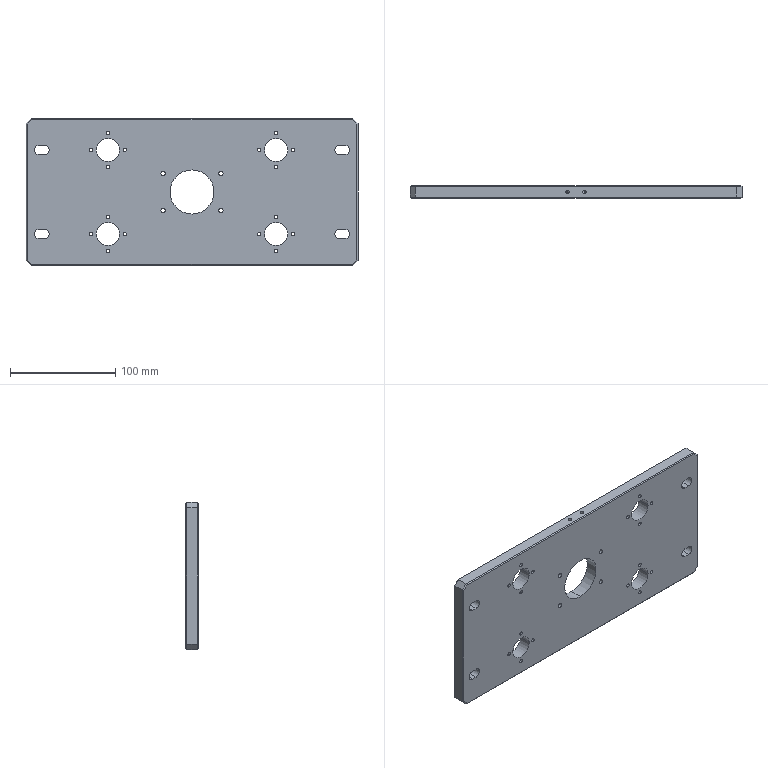Part | STEP file | BPSP-03-012 Linear Bearing Mounting Plate_Default | 1 solid | 108 faces | box 316 x 12 x 140 mm | volume 486609 mm3 | cylinder 66 | plane 34 | cone 8 | commonest cylinder face diameters 3.3 x40 4.2 x8 9 x8 22 x8 42 x2